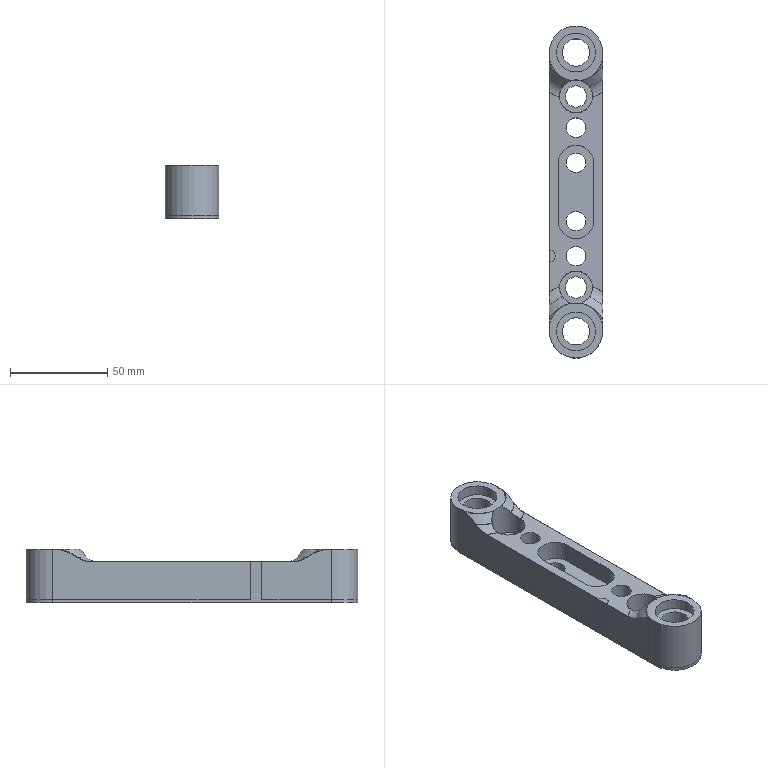NC program | NX | posted with a generic post | part box 27.4 x 170.48 x 27.5 mm
Lines 10722 to 10888 of 10888:
(PLANAR_MILL_1 , TOOL : D12精光)
N21394 T07 M6
N21396 G54
N21398 G17 G0 G90 X73.54 Y-21.9 B0. C0. S3500 M3
N21400 G43 Z30. H7
N21402 Z-29.
N21404 G94 G1 Z-31. F800.
N21406 G3 X71.54 Y-19.9 R2.
N21408 G1 X-71.54
N21410 G2 X-91.44 Y0. R19.9
N21412 X-71.54 Y19.9 R19.9
N21414 G1 X71.54
N21416 G2 X91.44 Y0. R19.9
N21418 X71.54 Y-19.9 R19.9
N21420 G3 X69.54 Y-21.9 R2.
N21422 G1 X73.54
N21424 G3 X71.54 Y-19.9 R2.
N21426 G1 X-71.54
N21428 G2 X-91.44 Y0. R19.9
N21430 X-71.54 Y19.9 R19.9
N21432 G1 X71.54
N21434 G2 X91.44 Y0. R19.9
N21436 X71.54 Y-19.9 R19.9
N21438 G3 X69.54 Y-21.9 R2.
N21440 G1 Z-29.
N21442 G0 Z30.
N21444 M5
(PLANAR_MILL_2 , TOOL : D8开粗)
N21446 T06 M6
N21448 G54
N21450 G17 G0 G90 X-49.137 Y-0.481 B0. C0. S3500 M3
N21452 G43 Z30. H6
N21454 Z-15.
N21456 G94 G1 Z-17. F500.
N21458 X-50. Y-3.5
N21460 G3 X-49. Y-4.5 R1.
N21462 X-44.5 Y0. R4.5
N21464 X-49. Y-4.5 R-4.5
N21466 X-48. Y-3.5 R1.
N21468 G1 X-50.
N21470 G3 X-49. Y-4.5 R1.
N21472 X-44.5 Y0. R4.5
N21474 X-49. Y-4.5 R-4.5
N21476 X-48. Y-3.5 R1.
N21478 G1 X-48.863 Y-0.481
N21480 Z-15.
N21482 G0 Z30.
N21484 X49.137 Y0.481
N21486 Z-15.
N21488 G1 Z-17.
N21490 X50. Y3.5
N21492 G3 X49. Y4.5 R1.
N21494 X44.5 Y0. R4.5
N21496 X49. Y4.5 R-4.5
N21498 X48. Y3.5 R1.
N21500 G1 X50.
N21502 G3 X49. Y4.5 R1.
N21504 X44.5 Y0. R4.5
N21506 X49. Y4.5 R-4.5
N21508 X48. Y3.5 R1.
N21510 G1 X48.863 Y0.481
N21512 Z-15.
N21514 G0 Z30.
N21516 M5
(PLANAR_MILL_3 , TOOL : D3倒角刀)
N21518 T09 M6
N21520 G54
N21522 G17 G0 G90 X-68.54 Y-16.8 B0. C0. S3500 M3
N21524 G43 Z30. H9
N21526 Z1.
N21528 G94 G1 Z-1. F800.
N21530 G3 X-70.54 Y-14.8 R2.
N21532 G1 X-71.54
N21534 G2 X-86.34 Y0. R14.8
N21536 X-71.54 Y14.8 R14.8
N21538 G1 X-70.54
N21540 G3 X-68.54 Y16.8 R2.
N21542 G1 Z1.
N21544 G0 Z30.
N21546 X68.54
N21548 Z1.
N21550 G1 Z-1.
N21552 G3 X70.54 Y14.8 R2.
N21554 G1 X71.54
N21556 G2 X86.34 Y0. R14.8
N21558 X71.54 Y-14.8 R14.8
N21560 G1 X70.54
N21562 G3 X68.54 Y-16.8 R2.
N21564 G1 Z1.
N21566 G0 Z30.
(PLANAR_MILL_3_COPY , TOOL : D3倒角刀)
N21568 X53.43
N21570 Z-5.5
N21572 G1 Z-7.5
N21574 G3 X51.43 Y-14.8 R2.
N21576 G1 X-51.43
N21578 G3 X-53.43 Y-16.8 R2.
N21580 G1 Z-5.5
N21582 G0 Z30.
N21584 Y16.8
N21586 Z-5.5
N21588 G1 Z-7.5
N21590 G3 X-51.43 Y14.8 R2.
N21592 G1 X51.43
N21594 G3 X53.43 Y16.8 R2.
N21596 G1 Z-5.5
N21598 G0 Z30.
(PLANAR_MILL_3_COPY_COPY , TOOL : D3倒角刀)
N21600 X-69.54 Y6.604
N21602 Z1.
N21604 G1 Z-1.
N21606 Y6.9
N21608 G3 X-71.54 Y8.9 R2.
N21610 X-80.44 Y0. R8.9
N21612 X-71.54 Y8.9 R-8.9
N21614 X-73.54 Y6.9 R2.
N21616 G1 Y6.604
N21618 Z1.
N21620 G0 Z30.
N21622 X69.54 Y-6.604
N21624 Z1.
N21626 G1 Z-1.
N21628 Y-6.9
N21630 G3 X71.54 Y-8.9 R2.
N21632 X80.44 Y0. R8.9
N21634 X71.54 Y-8.9 R-8.9
N21636 X73.54 Y-6.9 R2.
N21638 G1 Y-6.604
N21640 Z1.
N21642 G0 Z30.
(PLANAR_MILL_3_COPY_COPY_COPY , TOOL : D3倒角刀)
N21644 X-51. Y-1.5
N21646 Z-16.
N21648 G1 Z-18.
N21650 Y-2.5
N21652 G3 X-49. Y-4.5 R2.
N21654 X-44.5 Y0. R4.5
N21656 X-49. Y-4.5 R-4.5
N21658 X-47. Y-2.5 R2.
N21660 G1 Y-1.5
N21662 Z-16.
N21664 G0 Z30.
N21666 X47.
N21668 Z-16.
N21670 G1 Z-18.
N21672 Y-2.5
N21674 G3 X49. Y-4.5 R2.
N21676 X53.5 Y0. R4.5
N21678 X49. Y-4.5 R-4.5
N21680 X51. Y-2.5 R2.
N21682 G1 Y-1.5
N21684 Z-16.
N21686 G0 Z30.
N21688 M5
N21690 M2